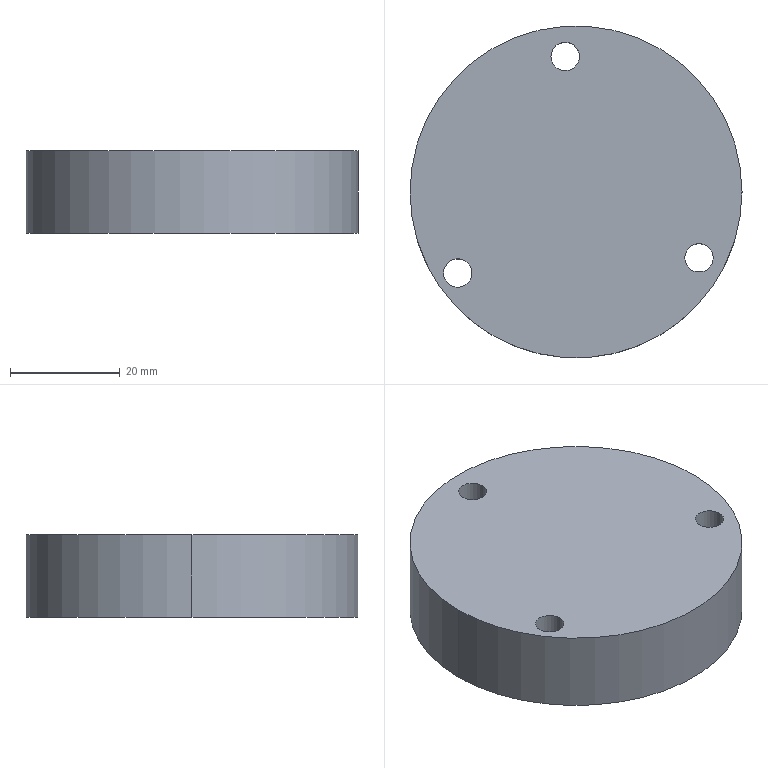Part | SolidWorks | features Extrusion 1 | 1 solid | 10 faces | box 60.454 x 60.454 x 15 mm | volume 42106 mm3 | cylinder 8 | plane 2 | commonest cylinder face diameters 5.182 x6 60.454 x2
STEP:
#1=CARTESIAN_POINT('',(5.015,-29.915,15.));
#2=VERTEX_POINT('',#1);
#3=CARTESIAN_POINT('',(10.197,-29.915,15.));
#4=VERTEX_POINT('',#3);
#5=CARTESIAN_POINT('',(7.606,-29.915,15.));
#6=DIRECTION('',(0.,0.,1.));
#7=DIRECTION('',(1.,0.,0.));
#8=AXIS2_PLACEMENT_3D('',#5,#6,#7);
#9=CIRCLE('',#8,2.591);
#10=EDGE_CURVE('',#2,#4,#9,.T.);
#11=ORIENTED_EDGE('',*,*,#10,.T.);
#12=CARTESIAN_POINT('',(10.197,-29.915,0.));
#13=VERTEX_POINT('',#12);
#14=CARTESIAN_POINT('',(10.197,-29.915,15.));
#15=DIRECTION('',(0.,0.,-1.));
#16=VECTOR('',#15,1000.);
#17=LINE('',#14,#16);
#18=EDGE_CURVE('',#4,#13,#17,.T.);
#19=ORIENTED_EDGE('',*,*,#18,.T.);
#20=CARTESIAN_POINT('',(5.015,-29.915,0.));
#21=VERTEX_POINT('',#20);
#22=CARTESIAN_POINT('',(7.606,-29.915,0.));
#23=DIRECTION('',(0.,0.,1.));
#24=DIRECTION('',(1.,0.,0.));
#25=AXIS2_PLACEMENT_3D('',#22,#23,#24);
#26=CIRCLE('',#25,2.591);
#27=EDGE_CURVE('',#21,#13,#26,.T.);
#28=ORIENTED_EDGE('',*,*,#27,.F.);
#29=CARTESIAN_POINT('',(5.015,-29.915,15.));
#30=DIRECTION('',(0.,0.,-1.));
#31=VECTOR('',#30,1000.);
#32=LINE('',#29,#31);
#33=EDGE_CURVE('',#2,#21,#32,.T.);
#34=ORIENTED_EDGE('',*,*,#33,.F.);
#35=EDGE_LOOP('',(#11,#19,#28,#34));
#36=FACE_OUTER_BOUND('',#35,.T.);
#37=CARTESIAN_POINT('',(7.606,-29.915,15.));
#38=DIRECTION('',(0.,0.,-1.));
#39=DIRECTION('',(-1.,0.,0.));
#40=AXIS2_PLACEMENT_3D('',#37,#38,#39);
#41=CYLINDRICAL_SURFACE('',#40,2.591);
#42=ADVANCED_FACE('',(#36),#41,.F.);
#43=CARTESIAN_POINT('',(-38.918,-32.687,15.));
#44=VERTEX_POINT('',#43);
#45=CARTESIAN_POINT('',(-33.736,-32.687,15.));
#46=VERTEX_POINT('',#45);
#47=CARTESIAN_POINT('',(-36.327,-32.687,15.));
#48=DIRECTION('',(0.,0.,1.));
#49=DIRECTION('',(1.,0.,0.));
#50=AXIS2_PLACEMENT_3D('',#47,#48,#49);
#51=CIRCLE('',#50,2.591);
#52=EDGE_CURVE('',#44,#46,#51,.T.);
#53=ORIENTED_EDGE('',*,*,#52,.T.);
#54=CARTESIAN_POINT('',(-33.736,-32.687,0.));
#55=VERTEX_POINT('',#54);
#56=CARTESIAN_POINT('',(-33.736,-32.687,15.));
#57=DIRECTION('',(0.,0.,-1.));
#58=VECTOR('',#57,1000.);
#59=LINE('',#56,#58);
#60=EDGE_CURVE('',#46,#55,#59,.T.);
#61=ORIENTED_EDGE('',*,*,#60,.T.);
#62=CARTESIAN_POINT('',(-38.918,-32.687,0.));
#63=VERTEX_POINT('',#62);
#64=CARTESIAN_POINT('',(-36.327,-32.687,0.));
#65=DIRECTION('',(0.,0.,1.));
#66=DIRECTION('',(1.,0.,0.));
#67=AXIS2_PLACEMENT_3D('',#64,#65,#66);
#68=CIRCLE('',#67,2.591);
#69=EDGE_CURVE('',#63,#55,#68,.T.);
#70=ORIENTED_EDGE('',*,*,#69,.F.);
#71=CARTESIAN_POINT('',(-38.918,-32.687,15.));
#72=DIRECTION('',(0.,0.,-1.));
#73=VECTOR('',#72,1000.);
#74=LINE('',#71,#73);
#75=EDGE_CURVE('',#44,#63,#74,.T.);
#76=ORIENTED_EDGE('',*,*,#75,.F.);
#77=EDGE_LOOP('',(#53,#61,#70,#76));
#78=FACE_OUTER_BOUND('',#77,.T.);
#79=CARTESIAN_POINT('',(-36.327,-32.687,15.));
#80=DIRECTION('',(0.,0.,-1.));
#81=DIRECTION('',(-1.,0.,0.));
#82=AXIS2_PLACEMENT_3D('',#79,#80,#81);
#83=CYLINDRICAL_SURFACE('',#82,2.591);
#84=ADVANCED_FACE('',(#78),#83,.F.);
#85=CARTESIAN_POINT('',(-19.352,6.746,15.));
#86=VERTEX_POINT('',#85);
#87=CARTESIAN_POINT('',(-14.17,6.746,15.));
#88=VERTEX_POINT('',#87);
#89=CARTESIAN_POINT('',(-16.761,6.746,15.));
#90=DIRECTION('',(0.,0.,1.));
#91=DIRECTION('',(1.,0.,0.));
#92=AXIS2_PLACEMENT_3D('',#89,#90,#91);
#93=CIRCLE('',#92,2.591);
#94=EDGE_CURVE('',#86,#88,#93,.T.);
#95=ORIENTED_EDGE('',*,*,#94,.T.);
#96=CARTESIAN_POINT('',(-14.17,6.746,0.));
#97=VERTEX_POINT('',#96);
#98=CARTESIAN_POINT('',(-14.17,6.746,15.));
#99=DIRECTION('',(0.,0.,-1.));
#100=VECTOR('',#99,1000.);
#101=LINE('',#98,#100);
#102=EDGE_CURVE('',#88,#97,#101,.T.);
#103=ORIENTED_EDGE('',*,*,#102,.T.);
#104=CARTESIAN_POINT('',(-19.352,6.746,0.));
#105=VERTEX_POINT('',#104);
#106=CARTESIAN_POINT('',(-16.761,6.746,0.));
#107=DIRECTION('',(0.,0.,1.));
#108=DIRECTION('',(1.,0.,0.));
#109=AXIS2_PLACEMENT_3D('',#106,#107,#108);
#110=CIRCLE('',#109,2.591);
#111=EDGE_CURVE('',#105,#97,#110,.T.);
#112=ORIENTED_EDGE('',*,*,#111,.F.);
#113=CARTESIAN_POINT('',(-19.352,6.746,15.));
#114=DIRECTION('',(0.,0.,-1.));
#115=VECTOR('',#114,1000.);
#116=LINE('',#113,#115);
#117=EDGE_CURVE('',#86,#105,#116,.T.);
#118=ORIENTED_EDGE('',*,*,#117,.F.);
#119=EDGE_LOOP('',(#95,#103,#112,#118));
#120=FACE_OUTER_BOUND('',#119,.T.);
#121=CARTESIAN_POINT('',(-16.761,6.746,15.));
#122=DIRECTION('',(0.,0.,-1.));
#123=DIRECTION('',(-1.,0.,0.));
#124=AXIS2_PLACEMENT_3D('',#121,#122,#123);
#125=CYLINDRICAL_SURFACE('',#124,2.591);
#126=ADVANCED_FACE('',(#120),#125,.F.);
#127=CARTESIAN_POINT('',(15.431,-17.915,15.));
#128=VERTEX_POINT('',#127);
#129=CARTESIAN_POINT('',(-45.022,-17.915,15.));
#130=VERTEX_POINT('',#129);
#131=CARTESIAN_POINT('',(-14.796,-17.915,15.));
#132=DIRECTION('',(0.,0.,1.));
#133=DIRECTION('',(1.,0.,0.));
#134=AXIS2_PLACEMENT_3D('',#131,#132,#133);
#135=CIRCLE('',#134,30.227);
#136=EDGE_CURVE('',#128,#130,#135,.T.);
#137=ORIENTED_EDGE('',*,*,#136,.F.);
#138=CARTESIAN_POINT('',(15.431,-17.915,0.));
#139=VERTEX_POINT('',#138);
#140=CARTESIAN_POINT('',(15.431,-17.915,15.));
#141=DIRECTION('',(0.,0.,-1.));
#142=VECTOR('',#141,1000.);
#143=LINE('',#140,#142);
#144=EDGE_CURVE('',#128,#139,#143,.T.);
#145=ORIENTED_EDGE('',*,*,#144,.T.);
#146=CARTESIAN_POINT('',(-45.022,-17.915,0.));
#147=VERTEX_POINT('',#146);
#148=CARTESIAN_POINT('',(-14.796,-17.915,0.));
#149=DIRECTION('',(0.,0.,1.));
#150=DIRECTION('',(1.,0.,0.));
#151=AXIS2_PLACEMENT_3D('',#148,#149,#150);
#152=CIRCLE('',#151,30.227);
#153=EDGE_CURVE('',#139,#147,#152,.T.);
#154=ORIENTED_EDGE('',*,*,#153,.T.);
#155=CARTESIAN_POINT('',(-45.022,-17.915,15.));
#156=DIRECTION('',(0.,0.,-1.));
#157=VECTOR('',#156,1000.);
#158=LINE('',#155,#157);
#159=EDGE_CURVE('',#130,#147,#158,.T.);
#160=ORIENTED_EDGE('',*,*,#159,.F.);
#161=EDGE_LOOP('',(#137,#145,#154,#160));
#162=FACE_OUTER_BOUND('',#161,.T.);
#163=CARTESIAN_POINT('',(-14.796,-17.915,15.));
#164=DIRECTION('',(0.,0.,-1.));
#165=DIRECTION('',(-1.,0.,0.));
#166=AXIS2_PLACEMENT_3D('',#163,#164,#165);
#167=CYLINDRICAL_SURFACE('',#166,30.227);
#168=ADVANCED_FACE('',(#162),#167,.T.);
#169=ORIENTED_EDGE('',*,*,#52,.F.);
#170=CARTESIAN_POINT('',(-36.327,-32.687,15.));
#171=DIRECTION('',(0.,0.,1.));
#172=DIRECTION('',(1.,0.,0.));
#173=AXIS2_PLACEMENT_3D('',#170,#171,#172);
#174=CIRCLE('',#173,2.591);
#175=EDGE_CURVE('',#46,#44,#174,.T.);
#176=ORIENTED_EDGE('',*,*,#175,.F.);
#177=EDGE_LOOP('',(#169,#176));
#178=FACE_BOUND('',#177,.T.);
#179=CARTESIAN_POINT('',(-14.796,-17.915,15.));
#180=DIRECTION('',(0.,0.,1.));
#181=DIRECTION('',(1.,0.,0.));
#182=AXIS2_PLACEMENT_3D('',#179,#180,#181);
#183=CIRCLE('',#182,30.227);
#184=EDGE_CURVE('',#130,#128,#183,.T.);
#185=ORIENTED_EDGE('',*,*,#184,.T.);
#186=ORIENTED_EDGE('',*,*,#136,.T.);
#187=EDGE_LOOP('',(#185,#186));
#188=FACE_OUTER_BOUND('',#187,.T.);
#189=ORIENTED_EDGE('',*,*,#94,.F.);
#190=CARTESIAN_POINT('',(-16.761,6.746,15.));
#191=DIRECTION('',(0.,0.,1.));
#192=DIRECTION('',(1.,0.,0.));
#193=AXIS2_PLACEMENT_3D('',#190,#191,#192);
#194=CIRCLE('',#193,2.591);
#195=EDGE_CURVE('',#88,#86,#194,.T.);
#196=ORIENTED_EDGE('',*,*,#195,.F.);
#197=EDGE_LOOP('',(#189,#196));
#198=FACE_BOUND('',#197,.T.);
#199=ORIENTED_EDGE('',*,*,#10,.F.);
#200=CARTESIAN_POINT('',(7.606,-29.915,15.));
#201=DIRECTION('',(0.,0.,1.));
#202=DIRECTION('',(1.,0.,0.));
#203=AXIS2_PLACEMENT_3D('',#200,#201,#202);
#204=CIRCLE('',#203,2.591);
#205=EDGE_CURVE('',#4,#2,#204,.T.);
#206=ORIENTED_EDGE('',*,*,#205,.F.);
#207=EDGE_LOOP('',(#199,#206));
#208=FACE_BOUND('',#207,.T.);
#209=CARTESIAN_POINT('',(-14.796,-17.915,15.));
#210=DIRECTION('',(0.,0.,1.));
#211=DIRECTION('',(1.,0.,0.));
#212=AXIS2_PLACEMENT_3D('',#209,#210,#211);
#213=PLANE('',#212);
#214=ADVANCED_FACE('',(#178,#188,#198,#208),#213,.T.);
#215=CARTESIAN_POINT('',(-14.796,-17.915,0.));
#216=DIRECTION('',(0.,0.,1.));
#217=DIRECTION('',(1.,0.,0.));
#218=AXIS2_PLACEMENT_3D('',#215,#216,#217);
#219=CIRCLE('',#218,30.227);
#220=EDGE_CURVE('',#147,#139,#219,.T.);
#221=ORIENTED_EDGE('',*,*,#220,.F.);
#222=ORIENTED_EDGE('',*,*,#153,.F.);
#223=EDGE_LOOP('',(#221,#222));
#224=FACE_OUTER_BOUND('',#223,.T.);
#225=ORIENTED_EDGE('',*,*,#111,.T.);
#226=CARTESIAN_POINT('',(-16.761,6.746,0.));
#227=DIRECTION('',(0.,0.,1.));
#228=DIRECTION('',(1.,0.,0.));
#229=AXIS2_PLACEMENT_3D('',#226,#227,#228);
#230=CIRCLE('',#229,2.591);
#231=EDGE_CURVE('',#97,#105,#230,.T.);
#232=ORIENTED_EDGE('',*,*,#231,.T.);
#233=EDGE_LOOP('',(#225,#232));
#234=FACE_BOUND('',#233,.T.);
#235=ORIENTED_EDGE('',*,*,#69,.T.);
#236=CARTESIAN_POINT('',(-36.327,-32.687,0.));
#237=DIRECTION('',(0.,0.,1.));
#238=DIRECTION('',(1.,0.,0.));
#239=AXIS2_PLACEMENT_3D('',#236,#237,#238);
#240=CIRCLE('',#239,2.591);
#241=EDGE_CURVE('',#55,#63,#240,.T.);
#242=ORIENTED_EDGE('',*,*,#241,.T.);
#243=EDGE_LOOP('',(#235,#242));
#244=FACE_BOUND('',#243,.T.);
#245=ORIENTED_EDGE('',*,*,#27,.T.);
#246=CARTESIAN_POINT('',(7.606,-29.915,0.));
#247=DIRECTION('',(0.,0.,1.));
#248=DIRECTION('',(1.,0.,0.));
#249=AXIS2_PLACEMENT_3D('',#246,#247,#248);
#250=CIRCLE('',#249,2.591);
#251=EDGE_CURVE('',#13,#21,#250,.T.);
#252=ORIENTED_EDGE('',*,*,#251,.T.);
#253=EDGE_LOOP('',(#245,#252));
#254=FACE_BOUND('',#253,.T.);
#255=CARTESIAN_POINT('',(-14.796,-17.915,0.));
#256=DIRECTION('',(0.,0.,1.));
#257=DIRECTION('',(1.,0.,0.));
#258=AXIS2_PLACEMENT_3D('',#255,#256,#257);
#259=PLANE('',#258);
#260=ADVANCED_FACE('',(#224,#234,#244,#254),#259,.F.);
#261=ORIENTED_EDGE('',*,*,#144,.F.);
#262=ORIENTED_EDGE('',*,*,#184,.F.);
#263=ORIENTED_EDGE('',*,*,#159,.T.);
#264=ORIENTED_EDGE('',*,*,#220,.T.);
#265=EDGE_LOOP('',(#261,#262,#263,#264));
#266=FACE_OUTER_BOUND('',#265,.T.);
#267=CARTESIAN_POINT('',(-14.796,-17.915,15.));
#268=DIRECTION('',(0.,0.,-1.));
#269=DIRECTION('',(-1.,0.,0.));
#270=AXIS2_PLACEMENT_3D('',#267,#268,#269);
#271=CYLINDRICAL_SURFACE('',#270,30.227);
#272=ADVANCED_FACE('',(#266),#271,.T.);
#273=ORIENTED_EDGE('',*,*,#102,.F.);
#274=ORIENTED_EDGE('',*,*,#195,.T.);
#275=ORIENTED_EDGE('',*,*,#117,.T.);
#276=ORIENTED_EDGE('',*,*,#231,.F.);
#277=EDGE_LOOP('',(#273,#274,#275,#276));
#278=FACE_OUTER_BOUND('',#277,.T.);
#279=CARTESIAN_POINT('',(-16.761,6.746,15.));
#280=DIRECTION('',(0.,0.,-1.));
#281=DIRECTION('',(-1.,0.,0.));
#282=AXIS2_PLACEMENT_3D('',#279,#280,#281);
#283=CYLINDRICAL_SURFACE('',#282,2.591);
#284=ADVANCED_FACE('',(#278),#283,.F.);
#285=ORIENTED_EDGE('',*,*,#60,.F.);
#286=ORIENTED_EDGE('',*,*,#175,.T.);
#287=ORIENTED_EDGE('',*,*,#75,.T.);
#288=ORIENTED_EDGE('',*,*,#241,.F.);
#289=EDGE_LOOP('',(#285,#286,#287,#288));
#290=FACE_OUTER_BOUND('',#289,.T.);
#291=CARTESIAN_POINT('',(-36.327,-32.687,15.));
#292=DIRECTION('',(0.,0.,-1.));
#293=DIRECTION('',(-1.,0.,0.));
#294=AXIS2_PLACEMENT_3D('',#291,#292,#293);
#295=CYLINDRICAL_SURFACE('',#294,2.591);
#296=ADVANCED_FACE('',(#290),#295,.F.);
#297=ORIENTED_EDGE('',*,*,#18,.F.);
#298=ORIENTED_EDGE('',*,*,#205,.T.);
#299=ORIENTED_EDGE('',*,*,#33,.T.);
#300=ORIENTED_EDGE('',*,*,#251,.F.);
#301=EDGE_LOOP('',(#297,#298,#299,#300));
#302=FACE_OUTER_BOUND('',#301,.T.);
#303=CARTESIAN_POINT('',(7.606,-29.915,15.));
#304=DIRECTION('',(0.,0.,-1.));
#305=DIRECTION('',(-1.,0.,0.));
#306=AXIS2_PLACEMENT_3D('',#303,#304,#305);
#307=CYLINDRICAL_SURFACE('',#306,2.591);
#308=ADVANCED_FACE('',(#302),#307,.F.);
#309=CLOSED_SHELL('',(#42,#84,#126,#168,#214,#260,#272,#284,#296,#308));
#310=MANIFOLD_SOLID_BREP('',#309);
#311=CARTESIAN_POINT('',(0.,0.,0.));
#312=DIRECTION('',(0.,0.,1.));
#313=DIRECTION('',(1.,0.,0.));
#314=AXIS2_PLACEMENT_3D('',#311,#312,#313);
#315=(LENGTH_UNIT()NAMED_UNIT(*)SI_UNIT(.MILLI.,.METRE.));
#316=UNCERTAINTY_MEASURE_WITH_UNIT(LENGTH_MEASURE(0.00001),#315,'','');
#317=(NAMED_UNIT(*)PLANE_ANGLE_UNIT()SI_UNIT($,.RADIAN.));
#318=(NAMED_UNIT(*)SI_UNIT($,.STERADIAN.)SOLID_ANGLE_UNIT());
#319=(GEOMETRIC_REPRESENTATION_CONTEXT(3)GLOBAL_UNCERTAINTY_ASSIGNED_CONTEXT((#316))GLOBAL_UNIT_ASSIGNED_CONTEXT((#315,#317,#318))REPRESENTATION_CONTEXT('',''));
#320=ADVANCED_BREP_SHAPE_REPRESENTATION('',(#310,#314),#319);